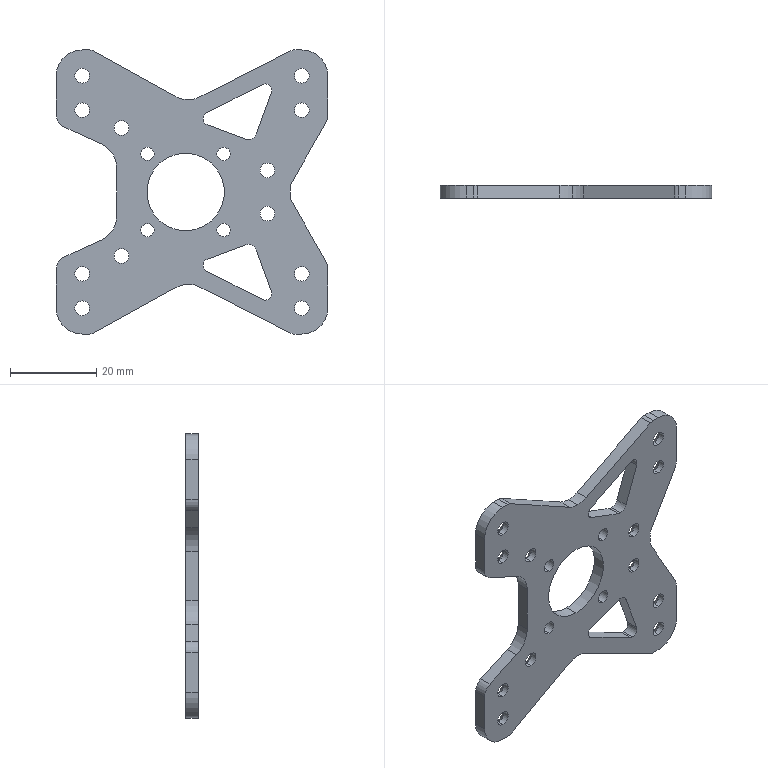Part | SolidWorks | features Fillet 5, ICE 2, Extrusion 1, HoleWzd 1 | 1 solid | 111 faces | box 63 x 3 x 66 mm | volume 7046 mm3 | cylinder 61 | plane 26 | cone 24 | commonest cylinder face diameters 3.4 x24 12 x9 3.1 x8 4 x7 6 x6 3 x5